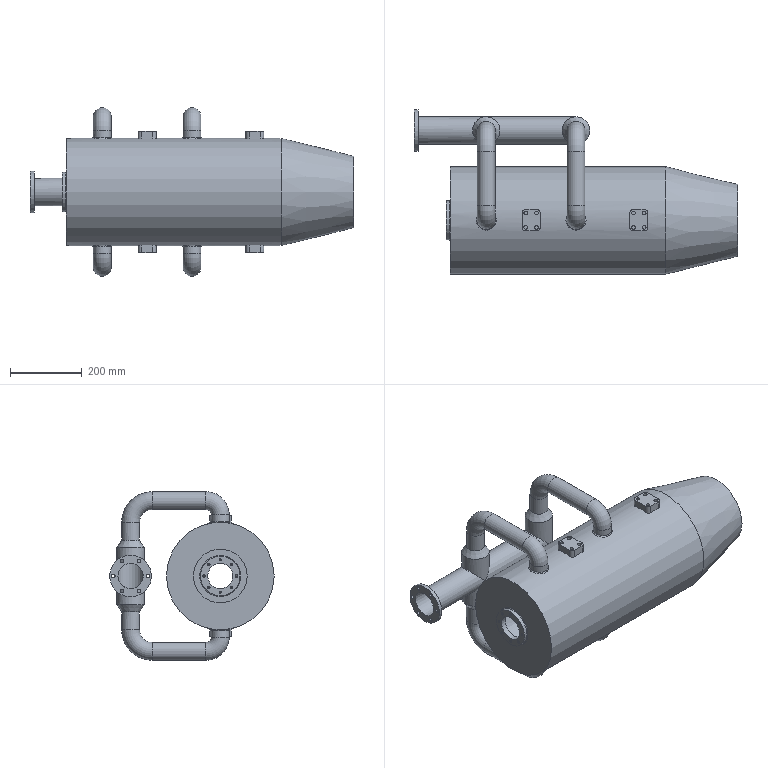Part | STEP file | Pulverized Coal Burner | 1 solid | 165 faces | box 900 x 458.1 x 470 mm | volume 45029265 mm3 | cylinder 84 | plane 42 | cone 18 | torus 17 | spline 4 | commonest cylinder face diameters 10 x22 20 x16 44 x12 50 x12 6.647 x8 70.2 x6